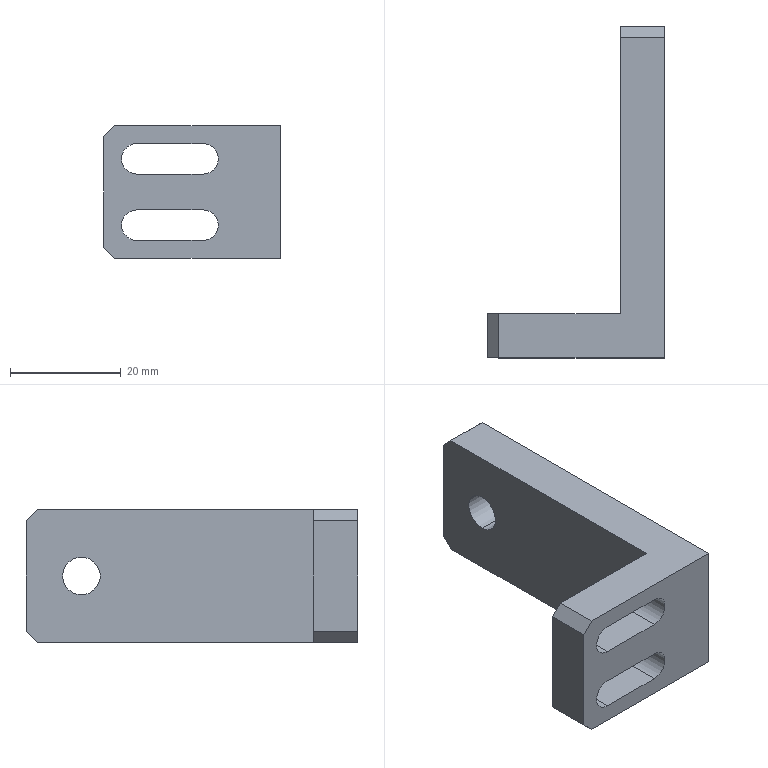Part | STEP file | 0-19 Buffer fixed 1 | 1 solid | 24 faces | box 32 x 60 x 24 mm | volume 14337 mm3 | plane 16 | cylinder 8 | commonest cylinder face diameters 5.5 x6 6.8 x2